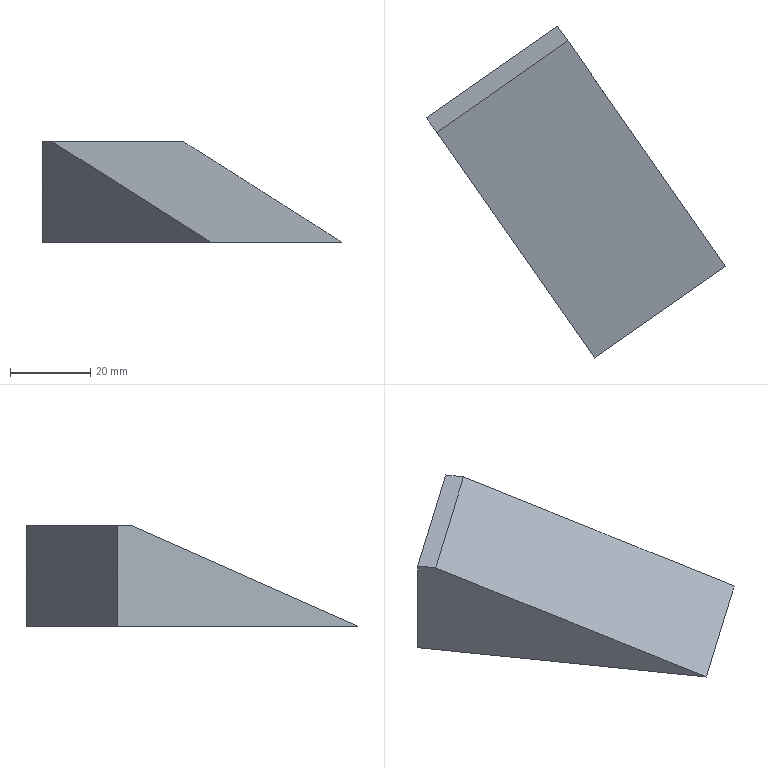Part | NX | features solid 2 | 1 solid | 6 faces | box 74.782 x 82.948 x 25 mm | volume 38909 mm3 | plane 6
STEP:
#1=CARTESIAN_POINT('',(-685.305,124.428,-19.));
#2=VERTEX_POINT('',#1);
#3=CARTESIAN_POINT('',(-685.305,124.428,-44.));
#4=VERTEX_POINT('',#3);
#5=CARTESIAN_POINT('',(-685.305,124.428,-19.));
#6=DIRECTION('',(0.,0.,-1.));
#7=VECTOR('',#6,1000.);
#8=LINE('',#5,#7);
#9=EDGE_CURVE('',#2,#4,#8,.T.);
#10=ORIENTED_EDGE('',*,*,#9,.T.);
#11=CARTESIAN_POINT('',(-718.071,101.485,-44.));
#12=VERTEX_POINT('',#11);
#13=CARTESIAN_POINT('',(-718.071,101.485,-44.));
#14=DIRECTION('',(0.8192,0.5736,0.));
#15=VECTOR('',#14,1000.);
#16=LINE('',#13,#15);
#17=EDGE_CURVE('',#12,#4,#16,.T.);
#18=ORIENTED_EDGE('',*,*,#17,.F.);
#19=CARTESIAN_POINT('',(-718.071,101.485,-19.));
#20=VERTEX_POINT('',#19);
#21=CARTESIAN_POINT('',(-718.071,101.485,-19.));
#22=DIRECTION('',(0.,0.,-1.));
#23=VECTOR('',#22,1000.);
#24=LINE('',#21,#23);
#25=EDGE_CURVE('',#20,#12,#24,.T.);
#26=ORIENTED_EDGE('',*,*,#25,.F.);
#27=CARTESIAN_POINT('',(-718.071,101.485,-19.));
#28=DIRECTION('',(0.8192,0.5736,0.));
#29=VECTOR('',#28,1000.);
#30=LINE('',#27,#29);
#31=EDGE_CURVE('',#20,#2,#30,.T.);
#32=ORIENTED_EDGE('',*,*,#31,.T.);
#33=EDGE_LOOP('',(#10,#18,#26,#32));
#34=FACE_BOUND('',#33,.T.);
#35=CARTESIAN_POINT('',(-718.071,101.485,-19.));
#36=DIRECTION('',(-0.5736,0.8192,0.));
#37=DIRECTION('',(0.8192,0.5736,0.));
#38=AXIS2_PLACEMENT_3D('',#35,#36,#37);
#39=PLANE('',#38);
#40=ADVANCED_FACE('',(#34),#39,.T.);
#41=CARTESIAN_POINT('',(-643.289,64.423,-44.));
#42=VERTEX_POINT('',#41);
#43=CARTESIAN_POINT('',(-643.289,64.423,-44.));
#44=DIRECTION('',(-0.5736,0.8192,0.));
#45=VECTOR('',#44,1000.);
#46=LINE('',#43,#45);
#47=EDGE_CURVE('',#42,#4,#46,.T.);
#48=ORIENTED_EDGE('',*,*,#47,.F.);
#49=CARTESIAN_POINT('',(-676.055,41.48,-44.));
#50=VERTEX_POINT('',#49);
#51=CARTESIAN_POINT('',(-676.055,41.48,-44.));
#52=DIRECTION('',(0.8192,0.5736,0.));
#53=VECTOR('',#52,1000.);
#54=LINE('',#51,#53);
#55=EDGE_CURVE('',#50,#42,#54,.T.);
#56=ORIENTED_EDGE('',*,*,#55,.F.);
#57=CARTESIAN_POINT('',(-676.055,41.48,-44.));
#58=DIRECTION('',(-0.5736,0.8192,0.));
#59=VECTOR('',#58,1000.);
#60=LINE('',#57,#59);
#61=EDGE_CURVE('',#50,#12,#60,.T.);
#62=ORIENTED_EDGE('',*,*,#61,.T.);
#63=ORIENTED_EDGE('',*,*,#17,.T.);
#64=EDGE_LOOP('',(#48,#56,#62,#63));
#65=FACE_BOUND('',#64,.T.);
#66=CARTESIAN_POINT('',(-676.055,41.48,-44.));
#67=DIRECTION('',(0.,0.,1.));
#68=DIRECTION('',(-0.5736,0.8192,0.));
#69=AXIS2_PLACEMENT_3D('',#66,#67,#68);
#70=PLANE('',#69);
#71=ADVANCED_FACE('',(#65),#70,.F.);
#72=CARTESIAN_POINT('',(-682.686,120.688,-19.));
#73=VERTEX_POINT('',#72);
#74=CARTESIAN_POINT('',(-682.686,120.688,-19.));
#75=DIRECTION('',(0.539,-0.7698,-0.342));
#76=VECTOR('',#75,1000.);
#77=LINE('',#74,#76);
#78=EDGE_CURVE('',#73,#42,#77,.T.);
#79=ORIENTED_EDGE('',*,*,#78,.F.);
#80=CARTESIAN_POINT('',(-715.452,97.745,-19.));
#81=VERTEX_POINT('',#80);
#82=CARTESIAN_POINT('',(-715.452,97.745,-19.));
#83=DIRECTION('',(0.8192,0.5736,0.));
#84=VECTOR('',#83,1000.);
#85=LINE('',#82,#84);
#86=EDGE_CURVE('',#81,#73,#85,.T.);
#87=ORIENTED_EDGE('',*,*,#86,.F.);
#88=CARTESIAN_POINT('',(-715.452,97.745,-19.));
#89=DIRECTION('',(0.539,-0.7698,-0.342));
#90=VECTOR('',#89,1000.);
#91=LINE('',#88,#90);
#92=EDGE_CURVE('',#81,#50,#91,.T.);
#93=ORIENTED_EDGE('',*,*,#92,.T.);
#94=ORIENTED_EDGE('',*,*,#55,.T.);
#95=EDGE_LOOP('',(#79,#87,#93,#94));
#96=FACE_BOUND('',#95,.T.);
#97=CARTESIAN_POINT('',(-715.452,97.745,-19.));
#98=DIRECTION('',(-0.1962,0.2802,-0.9397));
#99=DIRECTION('',(0.539,-0.7698,-0.342));
#100=AXIS2_PLACEMENT_3D('',#97,#98,#99);
#101=PLANE('',#100);
#102=ADVANCED_FACE('',(#96),#101,.F.);
#103=CARTESIAN_POINT('',(-685.305,124.428,-19.));
#104=DIRECTION('',(0.5736,-0.8192,0.));
#105=VECTOR('',#104,1000.);
#106=LINE('',#103,#105);
#107=EDGE_CURVE('',#2,#73,#106,.T.);
#108=ORIENTED_EDGE('',*,*,#107,.F.);
#109=ORIENTED_EDGE('',*,*,#31,.F.);
#110=CARTESIAN_POINT('',(-718.071,101.485,-19.));
#111=DIRECTION('',(0.5736,-0.8192,0.));
#112=VECTOR('',#111,1000.);
#113=LINE('',#110,#112);
#114=EDGE_CURVE('',#20,#81,#113,.T.);
#115=ORIENTED_EDGE('',*,*,#114,.T.);
#116=ORIENTED_EDGE('',*,*,#86,.T.);
#117=EDGE_LOOP('',(#108,#109,#115,#116));
#118=FACE_BOUND('',#117,.T.);
#119=CARTESIAN_POINT('',(-718.071,101.485,-19.));
#120=DIRECTION('',(0.,0.,-1.));
#121=DIRECTION('',(-0.8192,-0.5736,0.));
#122=AXIS2_PLACEMENT_3D('',#119,#120,#121);
#123=PLANE('',#122);
#124=ADVANCED_FACE('',(#118),#123,.F.);
#125=ORIENTED_EDGE('',*,*,#25,.T.);
#126=ORIENTED_EDGE('',*,*,#61,.F.);
#127=ORIENTED_EDGE('',*,*,#92,.F.);
#128=ORIENTED_EDGE('',*,*,#114,.F.);
#129=EDGE_LOOP('',(#125,#126,#127,#128));
#130=FACE_BOUND('',#129,.T.);
#131=CARTESIAN_POINT('',(-718.071,101.485,-19.));
#132=DIRECTION('',(0.8192,0.5736,0.));
#133=DIRECTION('',(0.5736,-0.8192,0.));
#134=AXIS2_PLACEMENT_3D('',#131,#132,#133);
#135=PLANE('',#134);
#136=ADVANCED_FACE('',(#130),#135,.F.);
#137=ORIENTED_EDGE('',*,*,#9,.F.);
#138=ORIENTED_EDGE('',*,*,#107,.T.);
#139=ORIENTED_EDGE('',*,*,#78,.T.);
#140=ORIENTED_EDGE('',*,*,#47,.T.);
#141=EDGE_LOOP('',(#137,#138,#139,#140));
#142=FACE_BOUND('',#141,.T.);
#143=CARTESIAN_POINT('',(-685.305,124.428,-19.));
#144=DIRECTION('',(0.8192,0.5736,0.));
#145=DIRECTION('',(0.5736,-0.8192,0.));
#146=AXIS2_PLACEMENT_3D('',#143,#144,#145);
#147=PLANE('',#146);
#148=ADVANCED_FACE('',(#142),#147,.T.);
#149=CLOSED_SHELL('',(#40,#71,#102,#124,#136,#148));
#150=MANIFOLD_SOLID_BREP('',#149);
#151=(LENGTH_UNIT()NAMED_UNIT(*)SI_UNIT(.MILLI.,.METRE.));
#152=UNCERTAINTY_MEASURE_WITH_UNIT(LENGTH_MEASURE(0.00001),#151,'','');
#153=(NAMED_UNIT(*)PLANE_ANGLE_UNIT()SI_UNIT($,.RADIAN.));
#154=(NAMED_UNIT(*)SI_UNIT($,.STERADIAN.)SOLID_ANGLE_UNIT());
#155=(GEOMETRIC_REPRESENTATION_CONTEXT(3)GLOBAL_UNCERTAINTY_ASSIGNED_CONTEXT((#152))GLOBAL_UNIT_ASSIGNED_CONTEXT((#151,#153,#154))REPRESENTATION_CONTEXT('',''));
#156=ADVANCED_BREP_SHAPE_REPRESENTATION('',(#150),#155);